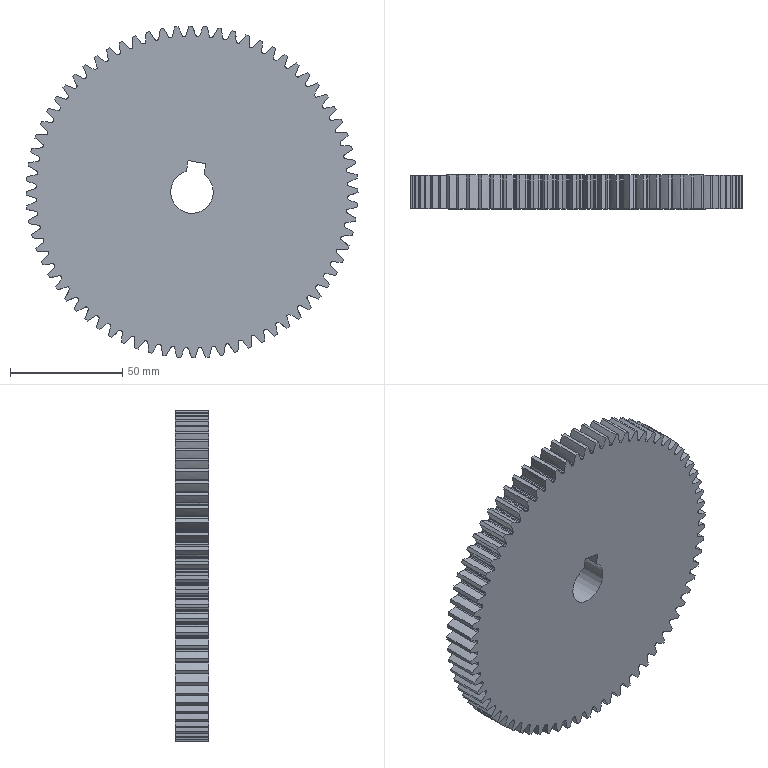Part | STEP file | 1_BODY_id914_x_t | 1 solid | 615 faces | box 148 x 15 x 148 mm | volume 238417 mm3 | other 465 | plane 77 | cylinder 73 | commonest cylinder face diameters 139 x72 19 x1